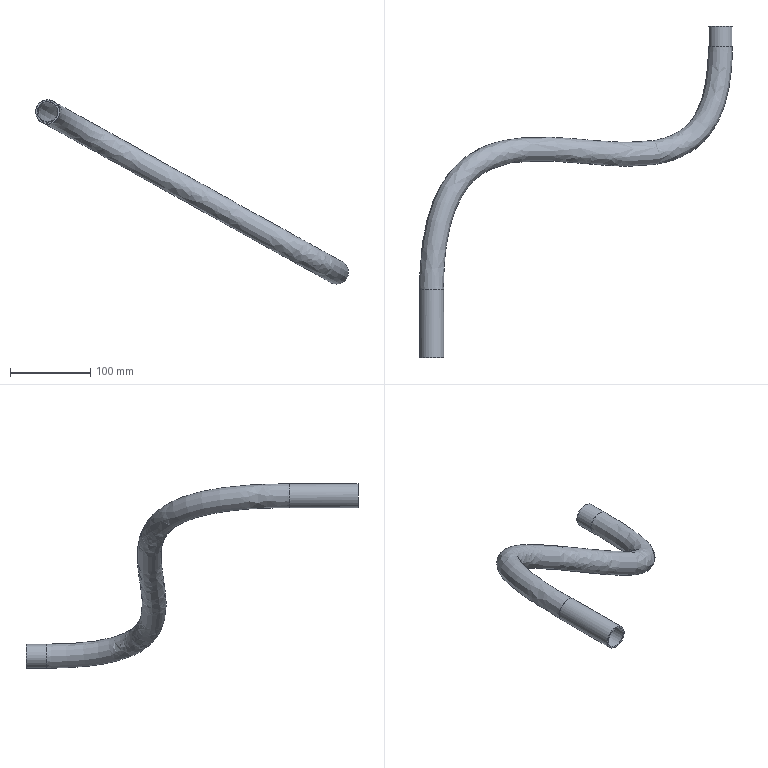Part | STEP file | Part 5^JBJ-F-0000-00 | 1 solid | 8 faces | box 391.028 x 414.992 x 230.424 mm | volume 128093 mm3 | cylinder 4 | spline 2 | plane 2 | commonest cylinder face diameters 26 x2 30 x2